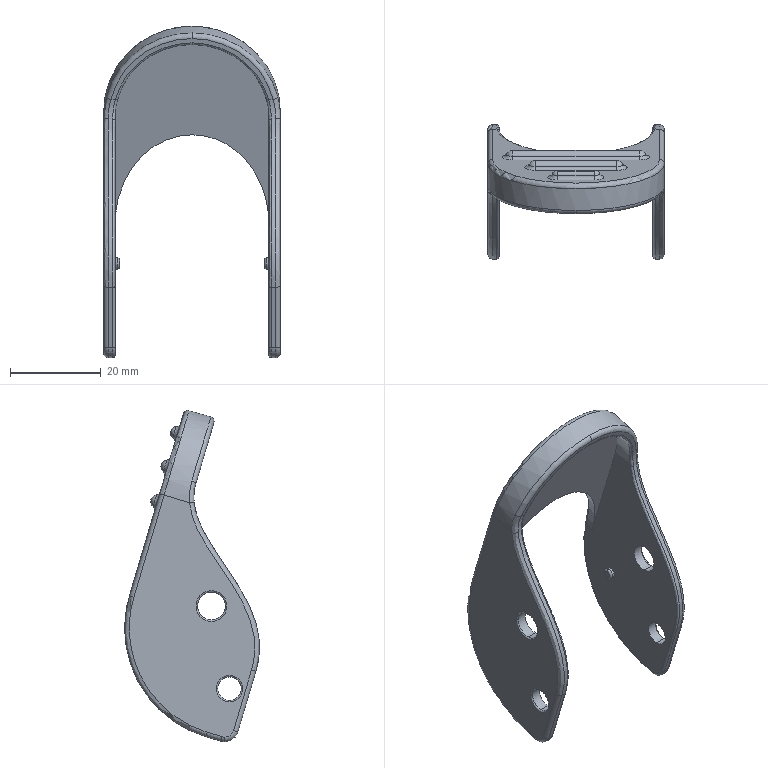Part | SolidWorks | features BaseBody 1 | 1 solid | 112 faces | box 39 x 29.721 x 73.171 mm | volume 8315 mm3 | cylinder 41 | torus 39 | plane 14 | spline 14 | sphere 4 | commonest cylinder face diameters 2 x15 1 x4 2.5 x4 5.2 x4 6.2 x4 3 x2